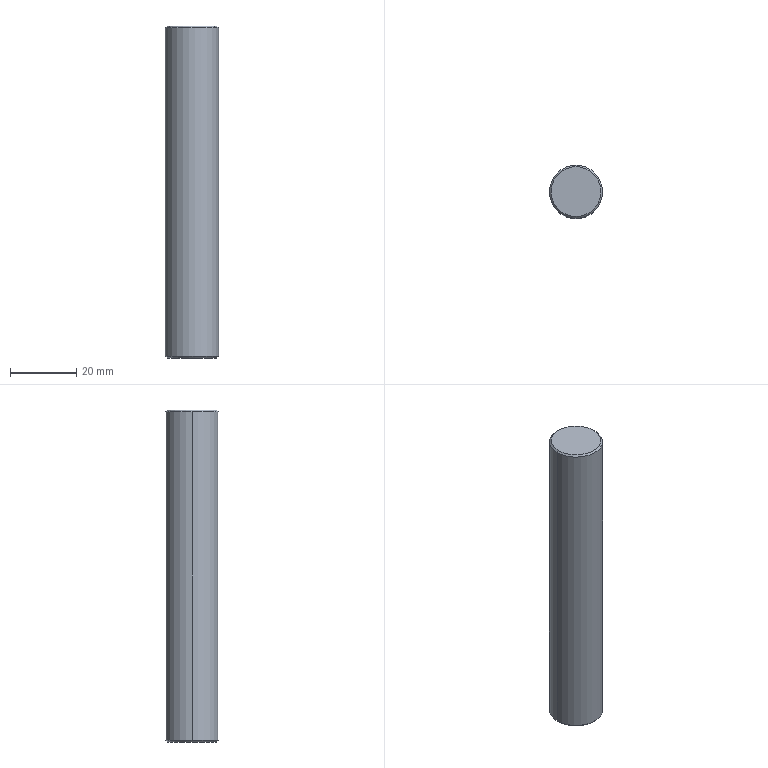Part | STEP file | X77-03205 | 1 solid | 8 faces | box 16 x 16 x 100 mm | volume 20094 mm3 | cone 4 | cylinder 2 | plane 2 | commonest cylinder face diameters 16 x2
STEP:
#1=CARTESIAN_POINT('',(7.5,0.,100.));
#2=VERTEX_POINT('',#1);
#3=CARTESIAN_POINT('',(-7.5,0.,100.));
#4=VERTEX_POINT('',#3);
#5=CARTESIAN_POINT('',(0.,0.,100.));
#6=DIRECTION('',(0.,0.,1.));
#7=DIRECTION('',(1.,0.,0.));
#8=AXIS2_PLACEMENT_3D('',#5,#6,#7);
#9=CIRCLE('',#8,7.5);
#10=EDGE_CURVE('',#2,#4,#9,.T.);
#11=ORIENTED_EDGE('',*,*,#10,.F.);
#12=CARTESIAN_POINT('',(8.,0.,99.5));
#13=VERTEX_POINT('',#12);
#14=CARTESIAN_POINT('',(7.5,0.,100.));
#15=DIRECTION('',(0.7071,0.,-0.7071));
#16=VECTOR('',#15,1000.);
#17=LINE('',#14,#16);
#18=EDGE_CURVE('',#2,#13,#17,.T.);
#19=ORIENTED_EDGE('',*,*,#18,.T.);
#20=CARTESIAN_POINT('',(-8.,0.,99.5));
#21=VERTEX_POINT('',#20);
#22=CARTESIAN_POINT('',(0.,0.,99.5));
#23=DIRECTION('',(0.,0.,-1.));
#24=DIRECTION('',(1.,0.,0.));
#25=AXIS2_PLACEMENT_3D('',#22,#23,#24);
#26=CIRCLE('',#25,8.);
#27=EDGE_CURVE('',#21,#13,#26,.T.);
#28=ORIENTED_EDGE('',*,*,#27,.F.);
#29=CARTESIAN_POINT('',(-7.5,0.,100.));
#30=DIRECTION('',(-0.7071,0.,-0.7071));
#31=VECTOR('',#30,1000.);
#32=LINE('',#29,#31);
#33=EDGE_CURVE('',#4,#21,#32,.T.);
#34=ORIENTED_EDGE('',*,*,#33,.F.);
#35=EDGE_LOOP('',(#11,#19,#28,#34));
#36=FACE_OUTER_BOUND('',#35,.T.);
#37=CARTESIAN_POINT('',(0.,0.,100.));
#38=DIRECTION('',(0.,0.,-1.));
#39=DIRECTION('',(-1.,0.,0.));
#40=AXIS2_PLACEMENT_3D('',#37,#38,#39);
#41=CONICAL_SURFACE('',#40,7.5,0.7854);
#42=ADVANCED_FACE('',(#36),#41,.T.);
#43=CARTESIAN_POINT('',(-7.5,0.,0.));
#44=VERTEX_POINT('',#43);
#45=CARTESIAN_POINT('',(7.5,0.,0.));
#46=VERTEX_POINT('',#45);
#47=CARTESIAN_POINT('',(0.,0.,0.));
#48=DIRECTION('',(0.,0.,-1.));
#49=DIRECTION('',(1.,0.,0.));
#50=AXIS2_PLACEMENT_3D('',#47,#48,#49);
#51=CIRCLE('',#50,7.5);
#52=EDGE_CURVE('',#44,#46,#51,.T.);
#53=ORIENTED_EDGE('',*,*,#52,.F.);
#54=CARTESIAN_POINT('',(-8.,0.,0.5));
#55=VERTEX_POINT('',#54);
#56=CARTESIAN_POINT('',(-8.,0.,0.5));
#57=DIRECTION('',(-0.7071,0.,0.7071));
#58=VECTOR('',#57,1000.);
#59=LINE('',#56,#58);
#60=EDGE_CURVE('',#44,#55,#59,.T.);
#61=ORIENTED_EDGE('',*,*,#60,.T.);
#62=CARTESIAN_POINT('',(8.,0.,0.5));
#63=VERTEX_POINT('',#62);
#64=CARTESIAN_POINT('',(0.,0.,0.5));
#65=DIRECTION('',(0.,0.,1.));
#66=DIRECTION('',(1.,0.,0.));
#67=AXIS2_PLACEMENT_3D('',#64,#65,#66);
#68=CIRCLE('',#67,8.);
#69=EDGE_CURVE('',#63,#55,#68,.T.);
#70=ORIENTED_EDGE('',*,*,#69,.F.);
#71=CARTESIAN_POINT('',(8.,0.,0.5));
#72=DIRECTION('',(0.7071,0.,0.7071));
#73=VECTOR('',#72,1000.);
#74=LINE('',#71,#73);
#75=EDGE_CURVE('',#46,#63,#74,.T.);
#76=ORIENTED_EDGE('',*,*,#75,.F.);
#77=EDGE_LOOP('',(#53,#61,#70,#76));
#78=FACE_OUTER_BOUND('',#77,.T.);
#79=CARTESIAN_POINT('',(0.,0.,0.5));
#80=DIRECTION('',(0.,0.,1.));
#81=DIRECTION('',(1.,0.,0.));
#82=AXIS2_PLACEMENT_3D('',#79,#80,#81);
#83=CONICAL_SURFACE('',#82,8.,0.7854);
#84=ADVANCED_FACE('',(#78),#83,.T.);
#85=ORIENTED_EDGE('',*,*,#27,.T.);
#86=CARTESIAN_POINT('',(8.,0.,100.));
#87=DIRECTION('',(0.,0.,-1.));
#88=VECTOR('',#87,1000.);
#89=LINE('',#86,#88);
#90=EDGE_CURVE('',#13,#63,#89,.T.);
#91=ORIENTED_EDGE('',*,*,#90,.T.);
#92=ORIENTED_EDGE('',*,*,#69,.T.);
#93=CARTESIAN_POINT('',(-8.,0.,100.));
#94=DIRECTION('',(0.,0.,-1.));
#95=VECTOR('',#94,1000.);
#96=LINE('',#93,#95);
#97=EDGE_CURVE('',#21,#55,#96,.T.);
#98=ORIENTED_EDGE('',*,*,#97,.F.);
#99=EDGE_LOOP('',(#85,#91,#92,#98));
#100=FACE_OUTER_BOUND('',#99,.T.);
#101=CARTESIAN_POINT('',(0.,0.,100.));
#102=DIRECTION('',(0.,0.,-1.));
#103=DIRECTION('',(-1.,0.,0.));
#104=AXIS2_PLACEMENT_3D('',#101,#102,#103);
#105=CYLINDRICAL_SURFACE('',#104,8.);
#106=ADVANCED_FACE('',(#100),#105,.T.);
#107=ORIENTED_EDGE('',*,*,#90,.F.);
#108=CARTESIAN_POINT('',(0.,0.,99.5));
#109=DIRECTION('',(0.,0.,-1.));
#110=DIRECTION('',(1.,0.,0.));
#111=AXIS2_PLACEMENT_3D('',#108,#109,#110);
#112=CIRCLE('',#111,8.);
#113=EDGE_CURVE('',#13,#21,#112,.T.);
#114=ORIENTED_EDGE('',*,*,#113,.T.);
#115=ORIENTED_EDGE('',*,*,#97,.T.);
#116=CARTESIAN_POINT('',(0.,0.,0.5));
#117=DIRECTION('',(0.,0.,1.));
#118=DIRECTION('',(1.,0.,0.));
#119=AXIS2_PLACEMENT_3D('',#116,#117,#118);
#120=CIRCLE('',#119,8.);
#121=EDGE_CURVE('',#55,#63,#120,.T.);
#122=ORIENTED_EDGE('',*,*,#121,.T.);
#123=EDGE_LOOP('',(#107,#114,#115,#122));
#124=FACE_OUTER_BOUND('',#123,.T.);
#125=CARTESIAN_POINT('',(0.,0.,100.));
#126=DIRECTION('',(0.,0.,-1.));
#127=DIRECTION('',(-1.,0.,0.));
#128=AXIS2_PLACEMENT_3D('',#125,#126,#127);
#129=CYLINDRICAL_SURFACE('',#128,8.);
#130=ADVANCED_FACE('',(#124),#129,.T.);
#131=CARTESIAN_POINT('',(0.,0.,100.));
#132=DIRECTION('',(0.,0.,1.));
#133=DIRECTION('',(1.,0.,0.));
#134=AXIS2_PLACEMENT_3D('',#131,#132,#133);
#135=CIRCLE('',#134,7.5);
#136=EDGE_CURVE('',#4,#2,#135,.T.);
#137=ORIENTED_EDGE('',*,*,#136,.T.);
#138=ORIENTED_EDGE('',*,*,#10,.T.);
#139=EDGE_LOOP('',(#137,#138));
#140=FACE_OUTER_BOUND('',#139,.T.);
#141=CARTESIAN_POINT('',(0.,0.,100.));
#142=DIRECTION('',(0.,0.,1.));
#143=DIRECTION('',(1.,0.,0.));
#144=AXIS2_PLACEMENT_3D('',#141,#142,#143);
#145=PLANE('',#144);
#146=ADVANCED_FACE('',(#140),#145,.T.);
#147=CARTESIAN_POINT('',(0.,0.,0.));
#148=DIRECTION('',(0.,0.,-1.));
#149=DIRECTION('',(1.,0.,0.));
#150=AXIS2_PLACEMENT_3D('',#147,#148,#149);
#151=CIRCLE('',#150,7.5);
#152=EDGE_CURVE('',#46,#44,#151,.T.);
#153=ORIENTED_EDGE('',*,*,#152,.T.);
#154=ORIENTED_EDGE('',*,*,#52,.T.);
#155=EDGE_LOOP('',(#153,#154));
#156=FACE_OUTER_BOUND('',#155,.T.);
#157=CARTESIAN_POINT('',(0.,0.,0.));
#158=DIRECTION('',(0.,0.,1.));
#159=DIRECTION('',(1.,0.,0.));
#160=AXIS2_PLACEMENT_3D('',#157,#158,#159);
#161=PLANE('',#160);
#162=ADVANCED_FACE('',(#156),#161,.F.);
#163=ORIENTED_EDGE('',*,*,#60,.F.);
#164=ORIENTED_EDGE('',*,*,#152,.F.);
#165=ORIENTED_EDGE('',*,*,#75,.T.);
#166=ORIENTED_EDGE('',*,*,#121,.F.);
#167=EDGE_LOOP('',(#163,#164,#165,#166));
#168=FACE_OUTER_BOUND('',#167,.T.);
#169=CARTESIAN_POINT('',(0.,0.,0.5));
#170=DIRECTION('',(0.,0.,1.));
#171=DIRECTION('',(1.,0.,0.));
#172=AXIS2_PLACEMENT_3D('',#169,#170,#171);
#173=CONICAL_SURFACE('',#172,8.,0.7854);
#174=ADVANCED_FACE('',(#168),#173,.T.);
#175=ORIENTED_EDGE('',*,*,#18,.F.);
#176=ORIENTED_EDGE('',*,*,#136,.F.);
#177=ORIENTED_EDGE('',*,*,#33,.T.);
#178=ORIENTED_EDGE('',*,*,#113,.F.);
#179=EDGE_LOOP('',(#175,#176,#177,#178));
#180=FACE_OUTER_BOUND('',#179,.T.);
#181=CARTESIAN_POINT('',(0.,0.,100.));
#182=DIRECTION('',(0.,0.,-1.));
#183=DIRECTION('',(-1.,0.,0.));
#184=AXIS2_PLACEMENT_3D('',#181,#182,#183);
#185=CONICAL_SURFACE('',#184,7.5,0.7854);
#186=ADVANCED_FACE('',(#180),#185,.T.);
#187=CLOSED_SHELL('',(#42,#84,#106,#130,#146,#162,#174,#186));
#188=MANIFOLD_SOLID_BREP('',#187);
#189=CARTESIAN_POINT('',(0.,0.,0.));
#190=DIRECTION('',(0.,0.,1.));
#191=DIRECTION('',(1.,0.,0.));
#192=AXIS2_PLACEMENT_3D('',#189,#190,#191);
#193=(LENGTH_UNIT()NAMED_UNIT(*)SI_UNIT(.MILLI.,.METRE.));
#194=UNCERTAINTY_MEASURE_WITH_UNIT(LENGTH_MEASURE(0.00001),#193,'','');
#195=(NAMED_UNIT(*)PLANE_ANGLE_UNIT()SI_UNIT($,.RADIAN.));
#196=(NAMED_UNIT(*)SI_UNIT($,.STERADIAN.)SOLID_ANGLE_UNIT());
#197=(GEOMETRIC_REPRESENTATION_CONTEXT(3)GLOBAL_UNCERTAINTY_ASSIGNED_CONTEXT((#194))GLOBAL_UNIT_ASSIGNED_CONTEXT((#193,#195,#196))REPRESENTATION_CONTEXT('',''));
#198=ADVANCED_BREP_SHAPE_REPRESENTATION('',(#188,#192),#197);